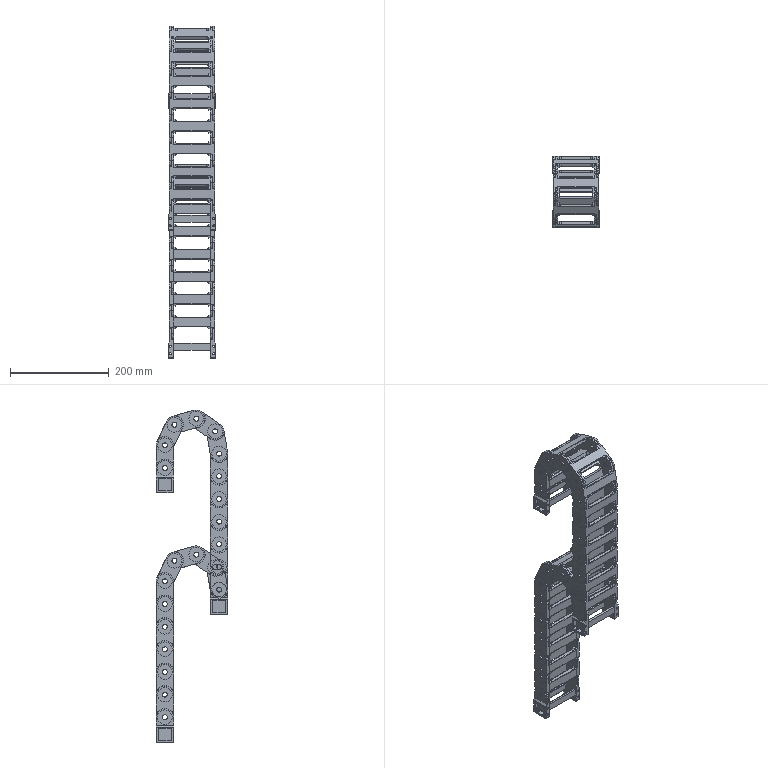Part | SolidWorks | features BaseBody 13, LPattern 3 | 24 solids | 5522 faces | volume 1022357 mm3 | cylinder 3000 | plane 2522 | commonest cylinder face diameters 2 x903 4.24 x252 18.2 x180 32.34 x174 10 x168 13.7 x168